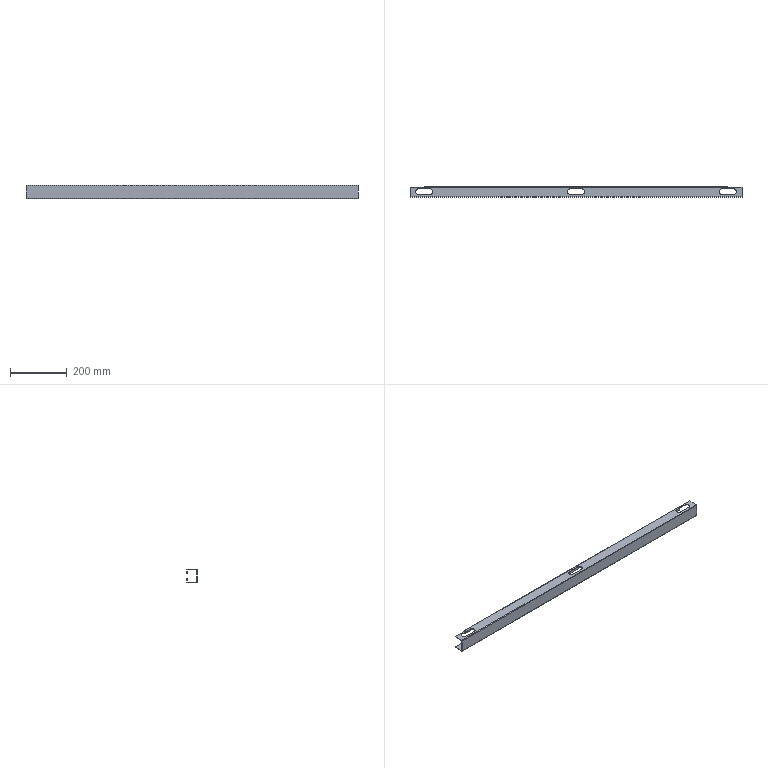Part | SolidWorks | features Cut 1, FlatPattern 1, ICE 1, SMBaseFlange 1, SheetMetal 1 | 1 solid | 70 faces | box 1169 x 38 x 46 mm | volume 238296 mm3 | plane 50 | cylinder 20 | commonest cylinder face diameters 20 x12 0.4 x4 3.4 x4